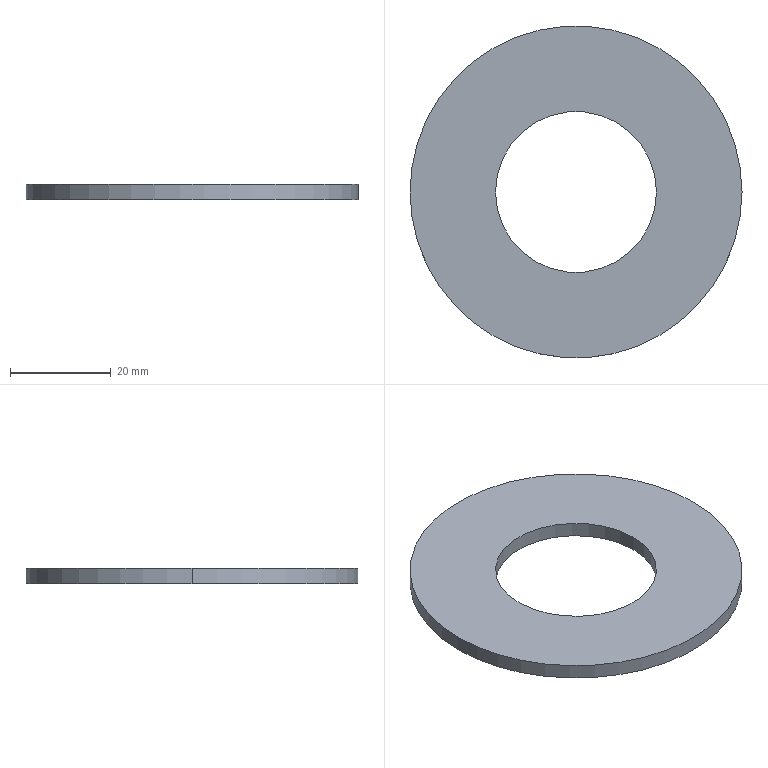Part | STEP file | 2089 Compression block A | 1 solid | 6 faces | box 66 x 66 x 3 mm | volume 7851 mm3 | cylinder 4 | plane 2 | commonest cylinder face diameters 32 x2 66 x2
STEP:
#1=CARTESIAN_POINT('',(0.,0.,0.));
#2=DIRECTION('',(0.,0.,1.));
#3=DIRECTION('',(1.,0.,0.));
#4=AXIS2_PLACEMENT_3D('',#1,#2,#3);
#5=CARTESIAN_POINT('',(-16.,0.,3.));
#6=VERTEX_POINT('',#5);
#7=CARTESIAN_POINT('',(-16.,0.,0.));
#8=VERTEX_POINT('',#7);
#9=CARTESIAN_POINT('',(-16.,0.,3.));
#10=DIRECTION('',(0.,0.,-1.));
#11=VECTOR('',#10,1.);
#12=LINE('',#9,#11);
#13=CARTESIAN_POINT('',(0.,0.,3.));
#14=DIRECTION('',(0.,0.,-1.));
#15=DIRECTION('',(-1.,0.,0.));
#16=AXIS2_PLACEMENT_3D('',#13,#14,#15);
#17=CYLINDRICAL_SURFACE('',#16,16.);
#18=CARTESIAN_POINT('',(6.283,0.));
#19=DIRECTION('',(0.,1.));
#20=VECTOR('',#19,1.);
#21=LINE('',#18,#20);
#22=(GEOMETRIC_REPRESENTATION_CONTEXT(2)PARAMETRIC_REPRESENTATION_CONTEXT()REPRESENTATION_CONTEXT('',''));
#23=DEFINITIONAL_REPRESENTATION('',(#21),#22);
#24=PCURVE('',#17,#23);
#25=CARTESIAN_POINT('',(0.,0.,3.));
#26=DIRECTION('',(0.,0.,-1.));
#27=DIRECTION('',(-1.,0.,0.));
#28=AXIS2_PLACEMENT_3D('',#25,#26,#27);
#29=CYLINDRICAL_SURFACE('',#28,16.);
#30=CARTESIAN_POINT('',(0.,0.));
#31=DIRECTION('',(0.,1.));
#32=VECTOR('',#31,1.);
#33=LINE('',#30,#32);
#34=(GEOMETRIC_REPRESENTATION_CONTEXT(2)PARAMETRIC_REPRESENTATION_CONTEXT()REPRESENTATION_CONTEXT('',''));
#35=DEFINITIONAL_REPRESENTATION('',(#33),#34);
#36=PCURVE('',#29,#35);
#37=SURFACE_CURVE('',#12,(#24,#36),.PCURVE_S1.);
#38=EDGE_CURVE('',#6,#8,#37,.T.);
#39=ORIENTED_EDGE('',*,*,#38,.T.);
#40=CARTESIAN_POINT('',(16.,0.,0.));
#41=VERTEX_POINT('',#40);
#42=CARTESIAN_POINT('',(0.,0.,0.));
#43=DIRECTION('',(0.,0.,1.));
#44=DIRECTION('',(1.,0.,0.));
#45=AXIS2_PLACEMENT_3D('',#42,#43,#44);
#46=CIRCLE('',#45,16.);
#47=CARTESIAN_POINT('',(9.425,3.));
#48=DIRECTION('',(-1.,0.));
#49=VECTOR('',#48,1.);
#50=LINE('',#47,#49);
#51=(GEOMETRIC_REPRESENTATION_CONTEXT(2)PARAMETRIC_REPRESENTATION_CONTEXT()REPRESENTATION_CONTEXT('',''));
#52=DEFINITIONAL_REPRESENTATION('',(#50),#51);
#53=PCURVE('',#17,#52);
#54=CARTESIAN_POINT('',(0.,0.,0.));
#55=DIRECTION('',(0.,0.,1.));
#56=DIRECTION('',(1.,0.,0.));
#57=AXIS2_PLACEMENT_3D('',#54,#55,#56);
#58=PLANE('',#57);
#59=CARTESIAN_POINT('',(0.,0.));
#60=DIRECTION('',(1.,0.));
#61=AXIS2_PLACEMENT_2D('',#59,#60);
#62=CIRCLE('',#61,16.);
#63=(GEOMETRIC_REPRESENTATION_CONTEXT(2)PARAMETRIC_REPRESENTATION_CONTEXT()REPRESENTATION_CONTEXT('',''));
#64=DEFINITIONAL_REPRESENTATION('',(#62),#63);
#65=PCURVE('',#58,#64);
#66=SURFACE_CURVE('',#46,(#53,#65),.PCURVE_S1.);
#67=EDGE_CURVE('',#8,#41,#66,.T.);
#68=ORIENTED_EDGE('',*,*,#67,.T.);
#69=CARTESIAN_POINT('',(16.,0.,3.));
#70=VERTEX_POINT('',#69);
#71=CARTESIAN_POINT('',(16.,0.,3.));
#72=DIRECTION('',(0.,0.,-1.));
#73=VECTOR('',#72,1.);
#74=LINE('',#71,#73);
#75=CARTESIAN_POINT('',(3.142,0.));
#76=DIRECTION('',(0.,1.));
#77=VECTOR('',#76,1.);
#78=LINE('',#75,#77);
#79=(GEOMETRIC_REPRESENTATION_CONTEXT(2)PARAMETRIC_REPRESENTATION_CONTEXT()REPRESENTATION_CONTEXT('',''));
#80=DEFINITIONAL_REPRESENTATION('',(#78),#79);
#81=PCURVE('',#17,#80);
#82=CARTESIAN_POINT('',(3.142,0.));
#83=DIRECTION('',(0.,1.));
#84=VECTOR('',#83,1.);
#85=LINE('',#82,#84);
#86=(GEOMETRIC_REPRESENTATION_CONTEXT(2)PARAMETRIC_REPRESENTATION_CONTEXT()REPRESENTATION_CONTEXT('',''));
#87=DEFINITIONAL_REPRESENTATION('',(#85),#86);
#88=PCURVE('',#29,#87);
#89=SURFACE_CURVE('',#74,(#81,#88),.PCURVE_S1.);
#90=EDGE_CURVE('',#70,#41,#89,.T.);
#91=ORIENTED_EDGE('',*,*,#90,.F.);
#92=CARTESIAN_POINT('',(0.,0.,3.));
#93=DIRECTION('',(0.,0.,1.));
#94=DIRECTION('',(1.,0.,0.));
#95=AXIS2_PLACEMENT_3D('',#92,#93,#94);
#96=CIRCLE('',#95,16.);
#97=CARTESIAN_POINT('',(9.425,0.));
#98=DIRECTION('',(-1.,0.));
#99=VECTOR('',#98,1.);
#100=LINE('',#97,#99);
#101=(GEOMETRIC_REPRESENTATION_CONTEXT(2)PARAMETRIC_REPRESENTATION_CONTEXT()REPRESENTATION_CONTEXT('',''));
#102=DEFINITIONAL_REPRESENTATION('',(#100),#101);
#103=PCURVE('',#17,#102);
#104=CARTESIAN_POINT('',(0.,0.,3.));
#105=DIRECTION('',(0.,0.,1.));
#106=DIRECTION('',(1.,0.,0.));
#107=AXIS2_PLACEMENT_3D('',#104,#105,#106);
#108=PLANE('',#107);
#109=CARTESIAN_POINT('',(0.,0.));
#110=DIRECTION('',(1.,0.));
#111=AXIS2_PLACEMENT_2D('',#109,#110);
#112=CIRCLE('',#111,16.);
#113=(GEOMETRIC_REPRESENTATION_CONTEXT(2)PARAMETRIC_REPRESENTATION_CONTEXT()REPRESENTATION_CONTEXT('',''));
#114=DEFINITIONAL_REPRESENTATION('',(#112),#113);
#115=PCURVE('',#108,#114);
#116=SURFACE_CURVE('',#96,(#103,#115),.PCURVE_S1.);
#117=EDGE_CURVE('',#6,#70,#116,.T.);
#118=ORIENTED_EDGE('',*,*,#117,.F.);
#119=EDGE_LOOP('',(#39,#68,#91,#118));
#120=FACE_BOUND('',#119,.F.);
#121=ADVANCED_FACE('',(#120),#17,.F.);
#122=CARTESIAN_POINT('',(33.,0.,3.));
#123=VERTEX_POINT('',#122);
#124=CARTESIAN_POINT('',(-33.,0.,3.));
#125=VERTEX_POINT('',#124);
#126=CARTESIAN_POINT('',(0.,0.,3.));
#127=DIRECTION('',(0.,0.,1.));
#128=DIRECTION('',(1.,0.,0.));
#129=AXIS2_PLACEMENT_3D('',#126,#127,#128);
#130=CIRCLE('',#129,33.);
#131=CARTESIAN_POINT('',(0.,0.,3.));
#132=DIRECTION('',(0.,0.,-1.));
#133=DIRECTION('',(-1.,0.,0.));
#134=AXIS2_PLACEMENT_3D('',#131,#132,#133);
#135=CYLINDRICAL_SURFACE('',#134,33.);
#136=CARTESIAN_POINT('',(3.142,0.));
#137=DIRECTION('',(-1.,0.));
#138=VECTOR('',#137,1.);
#139=LINE('',#136,#138);
#140=(GEOMETRIC_REPRESENTATION_CONTEXT(2)PARAMETRIC_REPRESENTATION_CONTEXT()REPRESENTATION_CONTEXT('',''));
#141=DEFINITIONAL_REPRESENTATION('',(#139),#140);
#142=PCURVE('',#135,#141);
#143=CARTESIAN_POINT('',(0.,0.));
#144=DIRECTION('',(1.,0.));
#145=AXIS2_PLACEMENT_2D('',#143,#144);
#146=CIRCLE('',#145,33.);
#147=(GEOMETRIC_REPRESENTATION_CONTEXT(2)PARAMETRIC_REPRESENTATION_CONTEXT()REPRESENTATION_CONTEXT('',''));
#148=DEFINITIONAL_REPRESENTATION('',(#146),#147);
#149=PCURVE('',#108,#148);
#150=SURFACE_CURVE('',#130,(#142,#149),.PCURVE_S1.);
#151=EDGE_CURVE('',#123,#125,#150,.T.);
#152=ORIENTED_EDGE('',*,*,#151,.F.);
#153=CARTESIAN_POINT('',(33.,0.,0.));
#154=VERTEX_POINT('',#153);
#155=CARTESIAN_POINT('',(33.,0.,3.));
#156=DIRECTION('',(0.,0.,-1.));
#157=VECTOR('',#156,1.);
#158=LINE('',#155,#157);
#159=CARTESIAN_POINT('',(3.142,0.));
#160=DIRECTION('',(0.,1.));
#161=VECTOR('',#160,1.);
#162=LINE('',#159,#161);
#163=(GEOMETRIC_REPRESENTATION_CONTEXT(2)PARAMETRIC_REPRESENTATION_CONTEXT()REPRESENTATION_CONTEXT('',''));
#164=DEFINITIONAL_REPRESENTATION('',(#162),#163);
#165=PCURVE('',#135,#164);
#166=CARTESIAN_POINT('',(0.,0.,3.));
#167=DIRECTION('',(0.,0.,-1.));
#168=DIRECTION('',(-1.,0.,0.));
#169=AXIS2_PLACEMENT_3D('',#166,#167,#168);
#170=CYLINDRICAL_SURFACE('',#169,33.);
#171=CARTESIAN_POINT('',(3.142,0.));
#172=DIRECTION('',(0.,1.));
#173=VECTOR('',#172,1.);
#174=LINE('',#171,#173);
#175=(GEOMETRIC_REPRESENTATION_CONTEXT(2)PARAMETRIC_REPRESENTATION_CONTEXT()REPRESENTATION_CONTEXT('',''));
#176=DEFINITIONAL_REPRESENTATION('',(#174),#175);
#177=PCURVE('',#170,#176);
#178=SURFACE_CURVE('',#158,(#165,#177),.PCURVE_S1.);
#179=EDGE_CURVE('',#123,#154,#178,.T.);
#180=ORIENTED_EDGE('',*,*,#179,.T.);
#181=CARTESIAN_POINT('',(-33.,0.,0.));
#182=VERTEX_POINT('',#181);
#183=CARTESIAN_POINT('',(0.,0.,0.));
#184=DIRECTION('',(0.,0.,1.));
#185=DIRECTION('',(1.,0.,0.));
#186=AXIS2_PLACEMENT_3D('',#183,#184,#185);
#187=CIRCLE('',#186,33.);
#188=CARTESIAN_POINT('',(3.142,3.));
#189=DIRECTION('',(-1.,0.));
#190=VECTOR('',#189,1.);
#191=LINE('',#188,#190);
#192=(GEOMETRIC_REPRESENTATION_CONTEXT(2)PARAMETRIC_REPRESENTATION_CONTEXT()REPRESENTATION_CONTEXT('',''));
#193=DEFINITIONAL_REPRESENTATION('',(#191),#192);
#194=PCURVE('',#135,#193);
#195=CARTESIAN_POINT('',(0.,0.));
#196=DIRECTION('',(1.,0.));
#197=AXIS2_PLACEMENT_2D('',#195,#196);
#198=CIRCLE('',#197,33.);
#199=(GEOMETRIC_REPRESENTATION_CONTEXT(2)PARAMETRIC_REPRESENTATION_CONTEXT()REPRESENTATION_CONTEXT('',''));
#200=DEFINITIONAL_REPRESENTATION('',(#198),#199);
#201=PCURVE('',#58,#200);
#202=SURFACE_CURVE('',#187,(#194,#201),.PCURVE_S1.);
#203=EDGE_CURVE('',#154,#182,#202,.T.);
#204=ORIENTED_EDGE('',*,*,#203,.T.);
#205=CARTESIAN_POINT('',(-33.,0.,3.));
#206=DIRECTION('',(0.,0.,-1.));
#207=VECTOR('',#206,1.);
#208=LINE('',#205,#207);
#209=CARTESIAN_POINT('',(0.,0.));
#210=DIRECTION('',(0.,1.));
#211=VECTOR('',#210,1.);
#212=LINE('',#209,#211);
#213=(GEOMETRIC_REPRESENTATION_CONTEXT(2)PARAMETRIC_REPRESENTATION_CONTEXT()REPRESENTATION_CONTEXT('',''));
#214=DEFINITIONAL_REPRESENTATION('',(#212),#213);
#215=PCURVE('',#135,#214);
#216=CARTESIAN_POINT('',(6.283,0.));
#217=DIRECTION('',(0.,1.));
#218=VECTOR('',#217,1.);
#219=LINE('',#216,#218);
#220=(GEOMETRIC_REPRESENTATION_CONTEXT(2)PARAMETRIC_REPRESENTATION_CONTEXT()REPRESENTATION_CONTEXT('',''));
#221=DEFINITIONAL_REPRESENTATION('',(#219),#220);
#222=PCURVE('',#170,#221);
#223=SURFACE_CURVE('',#208,(#215,#222),.PCURVE_S1.);
#224=EDGE_CURVE('',#125,#182,#223,.T.);
#225=ORIENTED_EDGE('',*,*,#224,.F.);
#226=EDGE_LOOP('',(#152,#180,#204,#225));
#227=FACE_BOUND('',#226,.T.);
#228=ADVANCED_FACE('',(#227),#135,.T.);
#229=CARTESIAN_POINT('',(0.,0.,3.));
#230=DIRECTION('',(0.,0.,1.));
#231=DIRECTION('',(1.,0.,0.));
#232=AXIS2_PLACEMENT_3D('',#229,#230,#231);
#233=CIRCLE('',#232,33.);
#234=CARTESIAN_POINT('',(0.,0.));
#235=DIRECTION('',(1.,0.));
#236=AXIS2_PLACEMENT_2D('',#234,#235);
#237=CIRCLE('',#236,33.);
#238=(GEOMETRIC_REPRESENTATION_CONTEXT(2)PARAMETRIC_REPRESENTATION_CONTEXT()REPRESENTATION_CONTEXT('',''));
#239=DEFINITIONAL_REPRESENTATION('',(#237),#238);
#240=PCURVE('',#108,#239);
#241=CARTESIAN_POINT('',(9.425,0.));
#242=DIRECTION('',(-1.,0.));
#243=VECTOR('',#242,1.);
#244=LINE('',#241,#243);
#245=(GEOMETRIC_REPRESENTATION_CONTEXT(2)PARAMETRIC_REPRESENTATION_CONTEXT()REPRESENTATION_CONTEXT('',''));
#246=DEFINITIONAL_REPRESENTATION('',(#244),#245);
#247=PCURVE('',#170,#246);
#248=SURFACE_CURVE('',#233,(#240,#247),.PCURVE_S1.);
#249=EDGE_CURVE('',#125,#123,#248,.T.);
#250=ORIENTED_EDGE('',*,*,#249,.T.);
#251=ORIENTED_EDGE('',*,*,#151,.T.);
#252=EDGE_LOOP('',(#250,#251));
#253=FACE_BOUND('',#252,.T.);
#254=ORIENTED_EDGE('',*,*,#117,.F.);
#255=CARTESIAN_POINT('',(0.,0.,3.));
#256=DIRECTION('',(0.,0.,1.));
#257=DIRECTION('',(1.,0.,0.));
#258=AXIS2_PLACEMENT_3D('',#255,#256,#257);
#259=CIRCLE('',#258,16.);
#260=CARTESIAN_POINT('',(0.,0.));
#261=DIRECTION('',(1.,0.));
#262=AXIS2_PLACEMENT_2D('',#260,#261);
#263=CIRCLE('',#262,16.);
#264=(GEOMETRIC_REPRESENTATION_CONTEXT(2)PARAMETRIC_REPRESENTATION_CONTEXT()REPRESENTATION_CONTEXT('',''));
#265=DEFINITIONAL_REPRESENTATION('',(#263),#264);
#266=PCURVE('',#108,#265);
#267=CARTESIAN_POINT('',(3.142,0.));
#268=DIRECTION('',(-1.,0.));
#269=VECTOR('',#268,1.);
#270=LINE('',#267,#269);
#271=(GEOMETRIC_REPRESENTATION_CONTEXT(2)PARAMETRIC_REPRESENTATION_CONTEXT()REPRESENTATION_CONTEXT('',''));
#272=DEFINITIONAL_REPRESENTATION('',(#270),#271);
#273=PCURVE('',#29,#272);
#274=SURFACE_CURVE('',#259,(#266,#273),.PCURVE_S1.);
#275=EDGE_CURVE('',#70,#6,#274,.T.);
#276=ORIENTED_EDGE('',*,*,#275,.F.);
#277=EDGE_LOOP('',(#254,#276));
#278=FACE_BOUND('',#277,.T.);
#279=ADVANCED_FACE('',(#253,#278),#108,.T.);
#280=CARTESIAN_POINT('',(0.,0.,0.));
#281=DIRECTION('',(0.,0.,1.));
#282=DIRECTION('',(1.,0.,0.));
#283=AXIS2_PLACEMENT_3D('',#280,#281,#282);
#284=CIRCLE('',#283,33.);
#285=CARTESIAN_POINT('',(0.,0.));
#286=DIRECTION('',(1.,0.));
#287=AXIS2_PLACEMENT_2D('',#285,#286);
#288=CIRCLE('',#287,33.);
#289=(GEOMETRIC_REPRESENTATION_CONTEXT(2)PARAMETRIC_REPRESENTATION_CONTEXT()REPRESENTATION_CONTEXT('',''));
#290=DEFINITIONAL_REPRESENTATION('',(#288),#289);
#291=PCURVE('',#58,#290);
#292=CARTESIAN_POINT('',(9.425,3.));
#293=DIRECTION('',(-1.,0.));
#294=VECTOR('',#293,1.);
#295=LINE('',#292,#294);
#296=(GEOMETRIC_REPRESENTATION_CONTEXT(2)PARAMETRIC_REPRESENTATION_CONTEXT()REPRESENTATION_CONTEXT('',''));
#297=DEFINITIONAL_REPRESENTATION('',(#295),#296);
#298=PCURVE('',#170,#297);
#299=SURFACE_CURVE('',#284,(#291,#298),.PCURVE_S1.);
#300=EDGE_CURVE('',#182,#154,#299,.T.);
#301=ORIENTED_EDGE('',*,*,#300,.F.);
#302=ORIENTED_EDGE('',*,*,#203,.F.);
#303=EDGE_LOOP('',(#301,#302));
#304=FACE_BOUND('',#303,.T.);
#305=ORIENTED_EDGE('',*,*,#67,.T.);
#306=CARTESIAN_POINT('',(0.,0.,0.));
#307=DIRECTION('',(0.,0.,1.));
#308=DIRECTION('',(1.,0.,0.));
#309=AXIS2_PLACEMENT_3D('',#306,#307,#308);
#310=CIRCLE('',#309,16.);
#311=CARTESIAN_POINT('',(0.,0.));
#312=DIRECTION('',(1.,0.));
#313=AXIS2_PLACEMENT_2D('',#311,#312);
#314=CIRCLE('',#313,16.);
#315=(GEOMETRIC_REPRESENTATION_CONTEXT(2)PARAMETRIC_REPRESENTATION_CONTEXT()REPRESENTATION_CONTEXT('',''));
#316=DEFINITIONAL_REPRESENTATION('',(#314),#315);
#317=PCURVE('',#58,#316);
#318=CARTESIAN_POINT('',(3.142,3.));
#319=DIRECTION('',(-1.,0.));
#320=VECTOR('',#319,1.);
#321=LINE('',#318,#320);
#322=(GEOMETRIC_REPRESENTATION_CONTEXT(2)PARAMETRIC_REPRESENTATION_CONTEXT()REPRESENTATION_CONTEXT('',''));
#323=DEFINITIONAL_REPRESENTATION('',(#321),#322);
#324=PCURVE('',#29,#323);
#325=SURFACE_CURVE('',#310,(#317,#324),.PCURVE_S1.);
#326=EDGE_CURVE('',#41,#8,#325,.T.);
#327=ORIENTED_EDGE('',*,*,#326,.T.);
#328=EDGE_LOOP('',(#305,#327));
#329=FACE_BOUND('',#328,.T.);
#330=ADVANCED_FACE('',(#304,#329),#58,.F.);
#331=ORIENTED_EDGE('',*,*,#179,.F.);
#332=ORIENTED_EDGE('',*,*,#249,.F.);
#333=ORIENTED_EDGE('',*,*,#224,.T.);
#334=ORIENTED_EDGE('',*,*,#300,.T.);
#335=EDGE_LOOP('',(#331,#332,#333,#334));
#336=FACE_BOUND('',#335,.T.);
#337=ADVANCED_FACE('',(#336),#170,.T.);
#338=ORIENTED_EDGE('',*,*,#326,.T.);
#339=ORIENTED_EDGE('',*,*,#38,.F.);
#340=ORIENTED_EDGE('',*,*,#275,.F.);
#341=ORIENTED_EDGE('',*,*,#90,.T.);
#342=EDGE_LOOP('',(#338,#339,#340,#341));
#343=FACE_BOUND('',#342,.F.);
#344=ADVANCED_FACE('',(#343),#29,.F.);
#345=CLOSED_SHELL('',(#121,#228,#279,#330,#337,#344));
#346=MANIFOLD_SOLID_BREP('',#345);
#347=(LENGTH_UNIT()NAMED_UNIT(*)SI_UNIT(.MILLI.,.METRE.));
#348=UNCERTAINTY_MEASURE_WITH_UNIT(LENGTH_MEASURE(0.0000001),#347,'','');
#349=(NAMED_UNIT(*)PLANE_ANGLE_UNIT()SI_UNIT($,.RADIAN.));
#350=(NAMED_UNIT(*)SI_UNIT($,.STERADIAN.)SOLID_ANGLE_UNIT());
#351=(GEOMETRIC_REPRESENTATION_CONTEXT(3)GLOBAL_UNCERTAINTY_ASSIGNED_CONTEXT((#348))GLOBAL_UNIT_ASSIGNED_CONTEXT((#347,#349,#350))REPRESENTATION_CONTEXT('',''));
#352=ADVANCED_BREP_SHAPE_REPRESENTATION('',(#4,#346),#351);